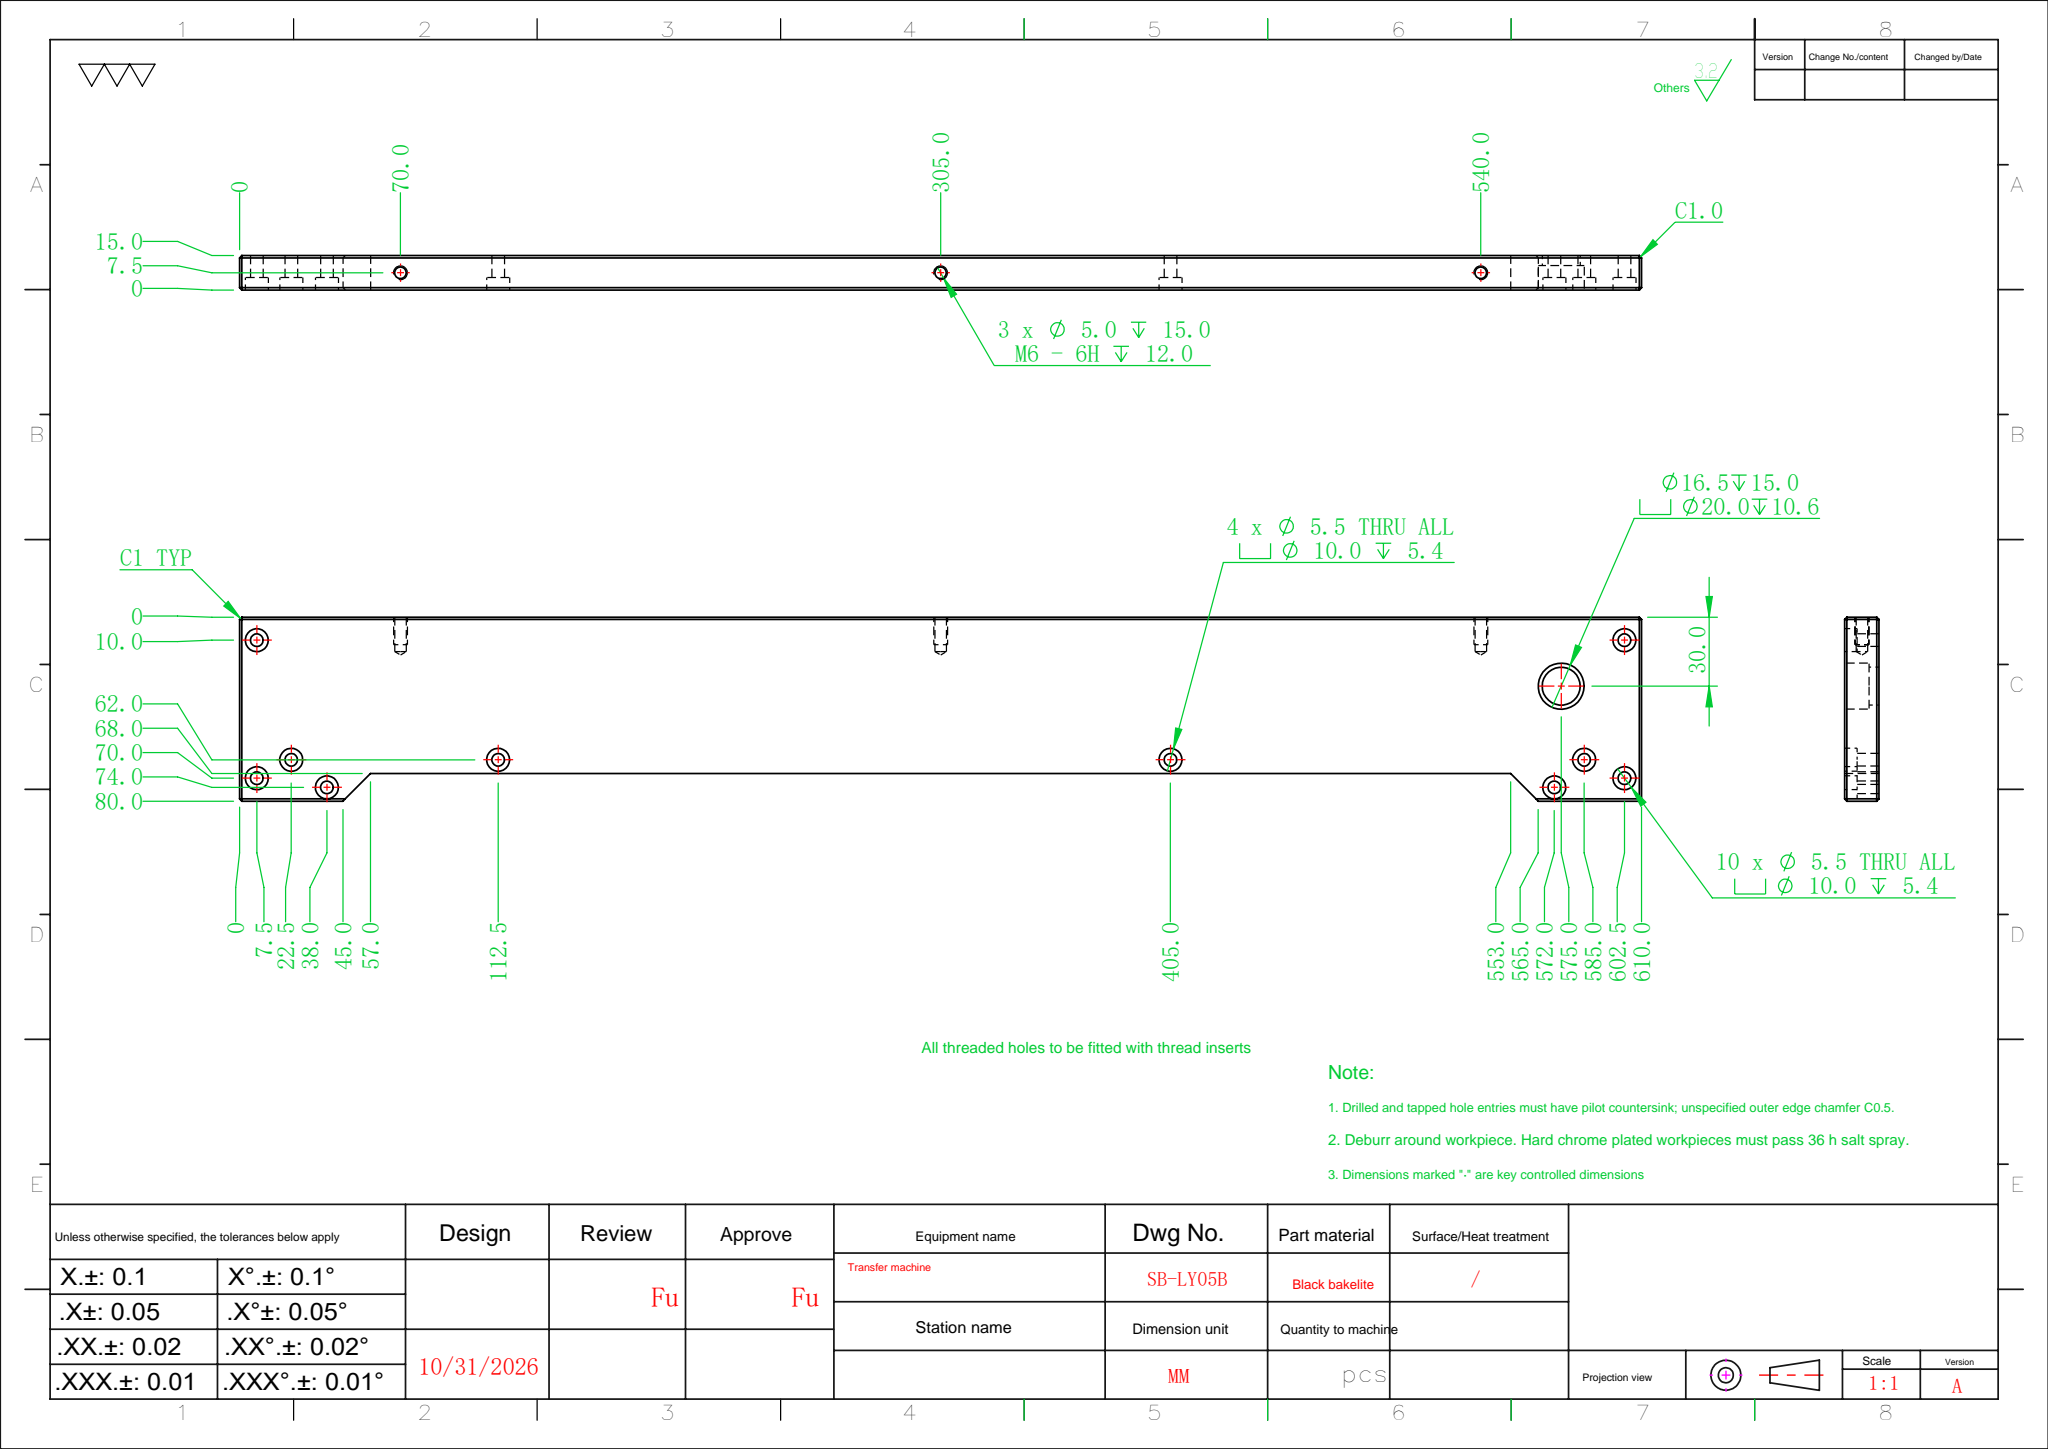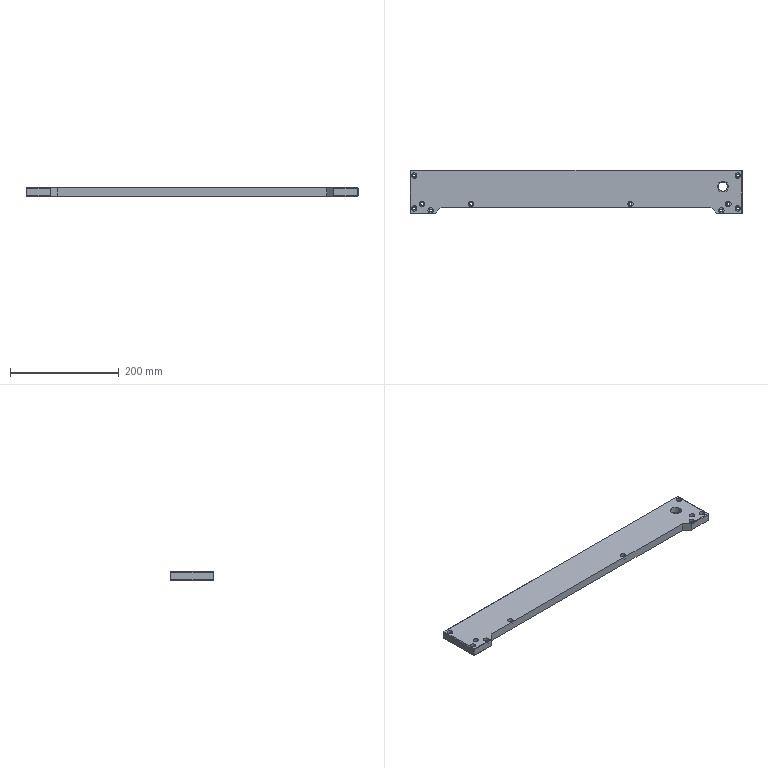Part | SolidWorks | features HoleWzd 4, Cut 3, Chamfer 2, Extrusion 1 | 1 solid | 99 faces | box 610 x 80 x 15 mm | volume 627969 mm3 | cylinder 50 | plane 43 | cone 6 | commonest cylinder face diameters 5.5 x20 10 x20 5 x6 16.5 x2 20 x2